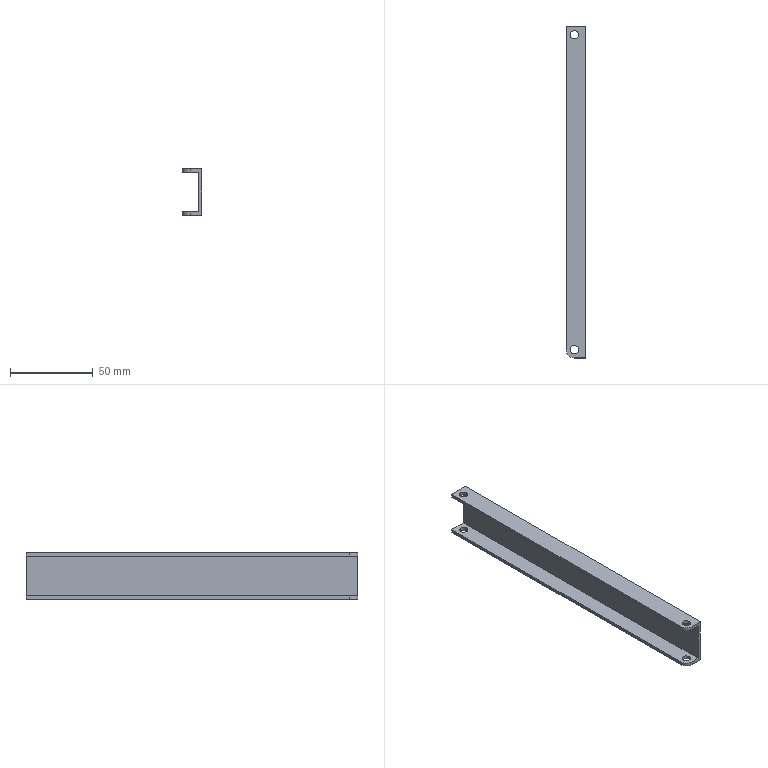Part | SolidWorks | features Cut 2, Extrusion 1, Fillet 1 | 1 solid | 20 faces | box 12 x 200 x 28 mm | volume 19021 mm3 | cylinder 10 | plane 10 | commonest cylinder face diameters 5 x8 10 x2
STEP:
#1=CARTESIAN_POINT('',(32.,242.23,-22.));
#2=VERTEX_POINT('',#1);
#3=CARTESIAN_POINT('',(32.,247.23,-22.));
#4=VERTEX_POINT('',#3);
#5=CARTESIAN_POINT('',(32.,244.73,-22.));
#6=DIRECTION('',(0.,0.,-1.));
#7=DIRECTION('',(-1.,0.,0.));
#8=AXIS2_PLACEMENT_3D('',#5,#6,#7);
#9=CIRCLE('',#8,2.5);
#10=EDGE_CURVE('',#2,#4,#9,.T.);
#11=ORIENTED_EDGE('',*,*,#10,.F.);
#12=CARTESIAN_POINT('',(32.,242.23,-24.));
#13=VERTEX_POINT('',#12);
#14=CARTESIAN_POINT('',(32.,242.23,4.));
#15=DIRECTION('',(0.,0.,-1.));
#16=VECTOR('',#15,1000.);
#17=LINE('',#14,#16);
#18=EDGE_CURVE('',#2,#13,#17,.T.);
#19=ORIENTED_EDGE('',*,*,#18,.T.);
#20=CARTESIAN_POINT('',(32.,247.23,-24.));
#21=VERTEX_POINT('',#20);
#22=CARTESIAN_POINT('',(32.,244.73,-24.));
#23=DIRECTION('',(0.,0.,-1.));
#24=DIRECTION('',(0.,1.,0.));
#25=AXIS2_PLACEMENT_3D('',#22,#23,#24);
#26=CIRCLE('',#25,2.5);
#27=EDGE_CURVE('',#13,#21,#26,.T.);
#28=ORIENTED_EDGE('',*,*,#27,.T.);
#29=CARTESIAN_POINT('',(32.,247.23,4.));
#30=DIRECTION('',(0.,0.,-1.));
#31=VECTOR('',#30,1000.);
#32=LINE('',#29,#31);
#33=EDGE_CURVE('',#4,#21,#32,.T.);
#34=ORIENTED_EDGE('',*,*,#33,.F.);
#35=EDGE_LOOP('',(#11,#19,#28,#34));
#36=FACE_OUTER_BOUND('',#35,.T.);
#37=CARTESIAN_POINT('',(32.,244.73,4.));
#38=DIRECTION('',(0.,0.,-1.));
#39=DIRECTION('',(0.,1.,0.));
#40=AXIS2_PLACEMENT_3D('',#37,#38,#39);
#41=CYLINDRICAL_SURFACE('',#40,2.5);
#42=ADVANCED_FACE('',(#36),#41,.F.);
#43=CARTESIAN_POINT('',(32.,242.23,4.));
#44=VERTEX_POINT('',#43);
#45=CARTESIAN_POINT('',(32.,247.23,4.));
#46=VERTEX_POINT('',#45);
#47=CARTESIAN_POINT('',(32.,244.73,4.));
#48=DIRECTION('',(0.,0.,-1.));
#49=DIRECTION('',(0.,1.,0.));
#50=AXIS2_PLACEMENT_3D('',#47,#48,#49);
#51=CIRCLE('',#50,2.5);
#52=EDGE_CURVE('',#44,#46,#51,.T.);
#53=ORIENTED_EDGE('',*,*,#52,.F.);
#54=CARTESIAN_POINT('',(32.,242.23,2.));
#55=VERTEX_POINT('',#54);
#56=CARTESIAN_POINT('',(32.,242.23,4.));
#57=DIRECTION('',(0.,0.,-1.));
#58=VECTOR('',#57,1000.);
#59=LINE('',#56,#58);
#60=EDGE_CURVE('',#44,#55,#59,.T.);
#61=ORIENTED_EDGE('',*,*,#60,.T.);
#62=CARTESIAN_POINT('',(32.,247.23,2.));
#63=VERTEX_POINT('',#62);
#64=CARTESIAN_POINT('',(32.,244.73,2.));
#65=DIRECTION('',(0.,0.,1.));
#66=DIRECTION('',(1.,0.,0.));
#67=AXIS2_PLACEMENT_3D('',#64,#65,#66);
#68=CIRCLE('',#67,2.5);
#69=EDGE_CURVE('',#63,#55,#68,.T.);
#70=ORIENTED_EDGE('',*,*,#69,.F.);
#71=CARTESIAN_POINT('',(32.,247.23,4.));
#72=DIRECTION('',(0.,0.,-1.));
#73=VECTOR('',#72,1000.);
#74=LINE('',#71,#73);
#75=EDGE_CURVE('',#46,#63,#74,.T.);
#76=ORIENTED_EDGE('',*,*,#75,.F.);
#77=EDGE_LOOP('',(#53,#61,#70,#76));
#78=FACE_OUTER_BOUND('',#77,.T.);
#79=CARTESIAN_POINT('',(32.,244.73,4.));
#80=DIRECTION('',(0.,0.,-1.));
#81=DIRECTION('',(0.,1.,0.));
#82=AXIS2_PLACEMENT_3D('',#79,#80,#81);
#83=CYLINDRICAL_SURFACE('',#82,2.5);
#84=ADVANCED_FACE('',(#78),#83,.F.);
#85=CARTESIAN_POINT('',(34.5,55.,-22.));
#86=VERTEX_POINT('',#85);
#87=CARTESIAN_POINT('',(29.5,55.,-22.));
#88=VERTEX_POINT('',#87);
#89=CARTESIAN_POINT('',(32.,55.,-22.));
#90=DIRECTION('',(0.,0.,-1.));
#91=DIRECTION('',(-1.,0.,0.));
#92=AXIS2_PLACEMENT_3D('',#89,#90,#91);
#93=CIRCLE('',#92,2.5);
#94=EDGE_CURVE('',#86,#88,#93,.T.);
#95=ORIENTED_EDGE('',*,*,#94,.F.);
#96=CARTESIAN_POINT('',(34.5,55.,-24.));
#97=VERTEX_POINT('',#96);
#98=CARTESIAN_POINT('',(34.5,55.,4.));
#99=DIRECTION('',(0.,0.,-1.));
#100=VECTOR('',#99,1000.);
#101=LINE('',#98,#100);
#102=EDGE_CURVE('',#86,#97,#101,.T.);
#103=ORIENTED_EDGE('',*,*,#102,.T.);
#104=CARTESIAN_POINT('',(29.5,55.,-24.));
#105=VERTEX_POINT('',#104);
#106=CARTESIAN_POINT('',(32.,55.,-24.));
#107=DIRECTION('',(0.,0.,-1.));
#108=DIRECTION('',(-1.,0.,0.));
#109=AXIS2_PLACEMENT_3D('',#106,#107,#108);
#110=CIRCLE('',#109,2.5);
#111=EDGE_CURVE('',#97,#105,#110,.T.);
#112=ORIENTED_EDGE('',*,*,#111,.T.);
#113=CARTESIAN_POINT('',(29.5,55.,4.));
#114=DIRECTION('',(0.,0.,-1.));
#115=VECTOR('',#114,1000.);
#116=LINE('',#113,#115);
#117=EDGE_CURVE('',#88,#105,#116,.T.);
#118=ORIENTED_EDGE('',*,*,#117,.F.);
#119=EDGE_LOOP('',(#95,#103,#112,#118));
#120=FACE_OUTER_BOUND('',#119,.T.);
#121=CARTESIAN_POINT('',(32.,55.,4.));
#122=DIRECTION('',(0.,0.,-1.));
#123=DIRECTION('',(-1.,0.,0.));
#124=AXIS2_PLACEMENT_3D('',#121,#122,#123);
#125=CYLINDRICAL_SURFACE('',#124,2.5);
#126=ADVANCED_FACE('',(#120),#125,.F.);
#127=CARTESIAN_POINT('',(34.5,55.,4.));
#128=VERTEX_POINT('',#127);
#129=CARTESIAN_POINT('',(29.5,55.,4.));
#130=VERTEX_POINT('',#129);
#131=CARTESIAN_POINT('',(32.,55.,4.));
#132=DIRECTION('',(0.,0.,-1.));
#133=DIRECTION('',(-1.,0.,0.));
#134=AXIS2_PLACEMENT_3D('',#131,#132,#133);
#135=CIRCLE('',#134,2.5);
#136=EDGE_CURVE('',#128,#130,#135,.T.);
#137=ORIENTED_EDGE('',*,*,#136,.F.);
#138=CARTESIAN_POINT('',(34.5,55.,2.));
#139=VERTEX_POINT('',#138);
#140=CARTESIAN_POINT('',(34.5,55.,4.));
#141=DIRECTION('',(0.,0.,-1.));
#142=VECTOR('',#141,1000.);
#143=LINE('',#140,#142);
#144=EDGE_CURVE('',#128,#139,#143,.T.);
#145=ORIENTED_EDGE('',*,*,#144,.T.);
#146=CARTESIAN_POINT('',(29.5,55.,2.));
#147=VERTEX_POINT('',#146);
#148=CARTESIAN_POINT('',(32.,55.,2.));
#149=DIRECTION('',(0.,0.,1.));
#150=DIRECTION('',(1.,0.,0.));
#151=AXIS2_PLACEMENT_3D('',#148,#149,#150);
#152=CIRCLE('',#151,2.5);
#153=EDGE_CURVE('',#147,#139,#152,.T.);
#154=ORIENTED_EDGE('',*,*,#153,.F.);
#155=CARTESIAN_POINT('',(29.5,55.,4.));
#156=DIRECTION('',(0.,0.,-1.));
#157=VECTOR('',#156,1000.);
#158=LINE('',#155,#157);
#159=EDGE_CURVE('',#130,#147,#158,.T.);
#160=ORIENTED_EDGE('',*,*,#159,.F.);
#161=EDGE_LOOP('',(#137,#145,#154,#160));
#162=FACE_OUTER_BOUND('',#161,.T.);
#163=CARTESIAN_POINT('',(32.,55.,4.));
#164=DIRECTION('',(0.,0.,-1.));
#165=DIRECTION('',(-1.,0.,0.));
#166=AXIS2_PLACEMENT_3D('',#163,#164,#165);
#167=CYLINDRICAL_SURFACE('',#166,2.5);
#168=ADVANCED_FACE('',(#162),#167,.F.);
#169=CARTESIAN_POINT('',(27.,250.,2.));
#170=VERTEX_POINT('',#169);
#171=CARTESIAN_POINT('',(27.,55.,2.));
#172=VERTEX_POINT('',#171);
#173=CARTESIAN_POINT('',(27.,250.,2.));
#174=DIRECTION('',(0.,-1.,0.));
#175=VECTOR('',#174,1000.);
#176=LINE('',#173,#175);
#177=EDGE_CURVE('',#170,#172,#176,.T.);
#178=ORIENTED_EDGE('',*,*,#177,.T.);
#179=CARTESIAN_POINT('',(27.,55.,4.));
#180=VERTEX_POINT('',#179);
#181=CARTESIAN_POINT('',(27.,55.,4.));
#182=DIRECTION('',(0.,0.,1.));
#183=VECTOR('',#182,1000.);
#184=LINE('',#181,#183);
#185=EDGE_CURVE('',#172,#180,#184,.T.);
#186=ORIENTED_EDGE('',*,*,#185,.T.);
#187=CARTESIAN_POINT('',(27.,250.,4.));
#188=VERTEX_POINT('',#187);
#189=CARTESIAN_POINT('',(27.,250.,4.));
#190=DIRECTION('',(0.,-1.,0.));
#191=VECTOR('',#190,1000.);
#192=LINE('',#189,#191);
#193=EDGE_CURVE('',#188,#180,#192,.T.);
#194=ORIENTED_EDGE('',*,*,#193,.F.);
#195=CARTESIAN_POINT('',(27.,250.,2.));
#196=DIRECTION('',(0.,0.,1.));
#197=VECTOR('',#196,1000.);
#198=LINE('',#195,#197);
#199=EDGE_CURVE('',#170,#188,#198,.T.);
#200=ORIENTED_EDGE('',*,*,#199,.F.);
#201=EDGE_LOOP('',(#178,#186,#194,#200));
#202=FACE_OUTER_BOUND('',#201,.T.);
#203=CARTESIAN_POINT('',(27.,250.,2.));
#204=DIRECTION('',(1.,0.,0.));
#205=DIRECTION('',(0.,0.,-1.));
#206=AXIS2_PLACEMENT_3D('',#203,#204,#205);
#207=PLANE('',#206);
#208=ADVANCED_FACE('',(#202),#207,.F.);
#209=CARTESIAN_POINT('',(32.,244.73,4.));
#210=DIRECTION('',(0.,0.,-1.));
#211=DIRECTION('',(0.,1.,0.));
#212=AXIS2_PLACEMENT_3D('',#209,#210,#211);
#213=CIRCLE('',#212,2.5);
#214=EDGE_CURVE('',#46,#44,#213,.T.);
#215=ORIENTED_EDGE('',*,*,#214,.T.);
#216=ORIENTED_EDGE('',*,*,#52,.T.);
#217=EDGE_LOOP('',(#215,#216));
#218=FACE_BOUND('',#217,.T.);
#219=CARTESIAN_POINT('',(32.,55.,4.));
#220=DIRECTION('',(0.,0.,-1.));
#221=DIRECTION('',(-1.,0.,0.));
#222=AXIS2_PLACEMENT_3D('',#219,#220,#221);
#223=CIRCLE('',#222,2.5);
#224=EDGE_CURVE('',#130,#128,#223,.T.);
#225=ORIENTED_EDGE('',*,*,#224,.T.);
#226=ORIENTED_EDGE('',*,*,#136,.T.);
#227=EDGE_LOOP('',(#225,#226));
#228=FACE_BOUND('',#227,.T.);
#229=ORIENTED_EDGE('',*,*,#193,.T.);
#230=CARTESIAN_POINT('',(32.,50.,4.));
#231=VERTEX_POINT('',#230);
#232=CARTESIAN_POINT('',(32.,55.,4.));
#233=DIRECTION('',(0.,0.,1.));
#234=DIRECTION('',(-1.,0.,0.));
#235=AXIS2_PLACEMENT_3D('',#232,#233,#234);
#236=CIRCLE('',#235,5.);
#237=EDGE_CURVE('',#180,#231,#236,.T.);
#238=ORIENTED_EDGE('',*,*,#237,.T.);
#239=CARTESIAN_POINT('',(39.,50.,4.));
#240=VERTEX_POINT('',#239);
#241=CARTESIAN_POINT('',(39.,50.,4.));
#242=DIRECTION('',(1.,0.,0.));
#243=VECTOR('',#242,1000.);
#244=LINE('',#241,#243);
#245=EDGE_CURVE('',#231,#240,#244,.T.);
#246=ORIENTED_EDGE('',*,*,#245,.T.);
#247=CARTESIAN_POINT('',(39.,250.,4.));
#248=VERTEX_POINT('',#247);
#249=CARTESIAN_POINT('',(39.,250.,4.));
#250=DIRECTION('',(0.,-1.,0.));
#251=VECTOR('',#250,1000.);
#252=LINE('',#249,#251);
#253=EDGE_CURVE('',#248,#240,#252,.T.);
#254=ORIENTED_EDGE('',*,*,#253,.F.);
#255=CARTESIAN_POINT('',(39.,250.,4.));
#256=DIRECTION('',(1.,0.,0.));
#257=VECTOR('',#256,1000.);
#258=LINE('',#255,#257);
#259=EDGE_CURVE('',#188,#248,#258,.T.);
#260=ORIENTED_EDGE('',*,*,#259,.F.);
#261=EDGE_LOOP('',(#229,#238,#246,#254,#260));
#262=FACE_OUTER_BOUND('',#261,.T.);
#263=CARTESIAN_POINT('',(39.,250.,4.));
#264=DIRECTION('',(0.,0.,-1.));
#265=DIRECTION('',(-1.,0.,0.));
#266=AXIS2_PLACEMENT_3D('',#263,#264,#265);
#267=PLANE('',#266);
#268=ADVANCED_FACE('',(#218,#228,#262),#267,.F.);
#269=CARTESIAN_POINT('',(39.,50.,-24.));
#270=VERTEX_POINT('',#269);
#271=CARTESIAN_POINT('',(39.,50.,-24.));
#272=DIRECTION('',(0.,0.,-1.));
#273=VECTOR('',#272,1000.);
#274=LINE('',#271,#273);
#275=EDGE_CURVE('',#240,#270,#274,.T.);
#276=ORIENTED_EDGE('',*,*,#275,.T.);
#277=CARTESIAN_POINT('',(39.,250.,-24.));
#278=VERTEX_POINT('',#277);
#279=CARTESIAN_POINT('',(39.,250.,-24.));
#280=DIRECTION('',(0.,-1.,0.));
#281=VECTOR('',#280,1000.);
#282=LINE('',#279,#281);
#283=EDGE_CURVE('',#278,#270,#282,.T.);
#284=ORIENTED_EDGE('',*,*,#283,.F.);
#285=CARTESIAN_POINT('',(39.,250.,-24.));
#286=DIRECTION('',(0.,0.,-1.));
#287=VECTOR('',#286,1000.);
#288=LINE('',#285,#287);
#289=EDGE_CURVE('',#248,#278,#288,.T.);
#290=ORIENTED_EDGE('',*,*,#289,.F.);
#291=ORIENTED_EDGE('',*,*,#253,.T.);
#292=EDGE_LOOP('',(#276,#284,#290,#291));
#293=FACE_OUTER_BOUND('',#292,.T.);
#294=CARTESIAN_POINT('',(39.,250.,-24.));
#295=DIRECTION('',(-1.,0.,0.));
#296=DIRECTION('',(0.,0.,1.));
#297=AXIS2_PLACEMENT_3D('',#294,#295,#296);
#298=PLANE('',#297);
#299=ADVANCED_FACE('',(#293),#298,.F.);
#300=CARTESIAN_POINT('',(32.,244.73,-24.));
#301=DIRECTION('',(0.,0.,-1.));
#302=DIRECTION('',(0.,1.,0.));
#303=AXIS2_PLACEMENT_3D('',#300,#301,#302);
#304=CIRCLE('',#303,2.5);
#305=EDGE_CURVE('',#21,#13,#304,.T.);
#306=ORIENTED_EDGE('',*,*,#305,.F.);
#307=ORIENTED_EDGE('',*,*,#27,.F.);
#308=EDGE_LOOP('',(#306,#307));
#309=FACE_BOUND('',#308,.T.);
#310=CARTESIAN_POINT('',(32.,55.,-24.));
#311=DIRECTION('',(0.,0.,-1.));
#312=DIRECTION('',(-1.,0.,0.));
#313=AXIS2_PLACEMENT_3D('',#310,#311,#312);
#314=CIRCLE('',#313,2.5);
#315=EDGE_CURVE('',#105,#97,#314,.T.);
#316=ORIENTED_EDGE('',*,*,#315,.F.);
#317=ORIENTED_EDGE('',*,*,#111,.F.);
#318=EDGE_LOOP('',(#316,#317));
#319=FACE_BOUND('',#318,.T.);
#320=CARTESIAN_POINT('',(32.,50.,-24.));
#321=VERTEX_POINT('',#320);
#322=CARTESIAN_POINT('',(27.,50.,-24.));
#323=DIRECTION('',(-1.,0.,0.));
#324=VECTOR('',#323,1000.);
#325=LINE('',#322,#324);
#326=EDGE_CURVE('',#270,#321,#325,.T.);
#327=ORIENTED_EDGE('',*,*,#326,.T.);
#328=CARTESIAN_POINT('',(27.,55.,-24.));
#329=VERTEX_POINT('',#328);
#330=CARTESIAN_POINT('',(32.,55.,-24.));
#331=DIRECTION('',(0.,0.,-1.));
#332=DIRECTION('',(1.,0.,0.));
#333=AXIS2_PLACEMENT_3D('',#330,#331,#332);
#334=CIRCLE('',#333,5.);
#335=EDGE_CURVE('',#321,#329,#334,.T.);
#336=ORIENTED_EDGE('',*,*,#335,.T.);
#337=CARTESIAN_POINT('',(27.,250.,-24.));
#338=VERTEX_POINT('',#337);
#339=CARTESIAN_POINT('',(27.,250.,-24.));
#340=DIRECTION('',(0.,-1.,0.));
#341=VECTOR('',#340,1000.);
#342=LINE('',#339,#341);
#343=EDGE_CURVE('',#338,#329,#342,.T.);
#344=ORIENTED_EDGE('',*,*,#343,.F.);
#345=CARTESIAN_POINT('',(27.,250.,-24.));
#346=DIRECTION('',(-1.,0.,0.));
#347=VECTOR('',#346,1000.);
#348=LINE('',#345,#347);
#349=EDGE_CURVE('',#278,#338,#348,.T.);
#350=ORIENTED_EDGE('',*,*,#349,.F.);
#351=ORIENTED_EDGE('',*,*,#283,.T.);
#352=EDGE_LOOP('',(#327,#336,#344,#350,#351));
#353=FACE_OUTER_BOUND('',#352,.T.);
#354=CARTESIAN_POINT('',(27.,250.,-24.));
#355=DIRECTION('',(0.,0.,1.));
#356=DIRECTION('',(1.,0.,0.));
#357=AXIS2_PLACEMENT_3D('',#354,#355,#356);
#358=PLANE('',#357);
#359=ADVANCED_FACE('',(#309,#319,#353),#358,.F.);
#360=ORIENTED_EDGE('',*,*,#343,.T.);
#361=CARTESIAN_POINT('',(27.,55.,-22.));
#362=VERTEX_POINT('',#361);
#363=CARTESIAN_POINT('',(27.,55.,-22.));
#364=DIRECTION('',(0.,0.,1.));
#365=VECTOR('',#364,1000.);
#366=LINE('',#363,#365);
#367=EDGE_CURVE('',#329,#362,#366,.T.);
#368=ORIENTED_EDGE('',*,*,#367,.T.);
#369=CARTESIAN_POINT('',(27.,250.,-22.));
#370=VERTEX_POINT('',#369);
#371=CARTESIAN_POINT('',(27.,250.,-22.));
#372=DIRECTION('',(0.,-1.,0.));
#373=VECTOR('',#372,1000.);
#374=LINE('',#371,#373);
#375=EDGE_CURVE('',#370,#362,#374,.T.);
#376=ORIENTED_EDGE('',*,*,#375,.F.);
#377=CARTESIAN_POINT('',(27.,250.,-22.));
#378=DIRECTION('',(0.,0.,1.));
#379=VECTOR('',#378,1000.);
#380=LINE('',#377,#379);
#381=EDGE_CURVE('',#338,#370,#380,.T.);
#382=ORIENTED_EDGE('',*,*,#381,.F.);
#383=EDGE_LOOP('',(#360,#368,#376,#382));
#384=FACE_OUTER_BOUND('',#383,.T.);
#385=CARTESIAN_POINT('',(27.,250.,-22.));
#386=DIRECTION('',(1.,0.,0.));
#387=DIRECTION('',(0.,0.,-1.));
#388=AXIS2_PLACEMENT_3D('',#385,#386,#387);
#389=PLANE('',#388);
#390=ADVANCED_FACE('',(#384),#389,.F.);
#391=CARTESIAN_POINT('',(32.,244.73,-22.));
#392=DIRECTION('',(0.,0.,-1.));
#393=DIRECTION('',(-1.,0.,0.));
#394=AXIS2_PLACEMENT_3D('',#391,#392,#393);
#395=CIRCLE('',#394,2.5);
#396=EDGE_CURVE('',#4,#2,#395,.T.);
#397=ORIENTED_EDGE('',*,*,#396,.T.);
#398=ORIENTED_EDGE('',*,*,#10,.T.);
#399=EDGE_LOOP('',(#397,#398));
#400=FACE_BOUND('',#399,.T.);
#401=CARTESIAN_POINT('',(32.,55.,-22.));
#402=DIRECTION('',(0.,0.,-1.));
#403=DIRECTION('',(-1.,0.,0.));
#404=AXIS2_PLACEMENT_3D('',#401,#402,#403);
#405=CIRCLE('',#404,2.5);
#406=EDGE_CURVE('',#88,#86,#405,.T.);
#407=ORIENTED_EDGE('',*,*,#406,.T.);
#408=ORIENTED_EDGE('',*,*,#94,.T.);
#409=EDGE_LOOP('',(#407,#408));
#410=FACE_BOUND('',#409,.T.);
#411=ORIENTED_EDGE('',*,*,#375,.T.);
#412=CARTESIAN_POINT('',(32.,50.,-22.));
#413=VERTEX_POINT('',#412);
#414=CARTESIAN_POINT('',(32.,55.,-22.));
#415=DIRECTION('',(0.,0.,1.));
#416=DIRECTION('',(-1.,0.,0.));
#417=AXIS2_PLACEMENT_3D('',#414,#415,#416);
#418=CIRCLE('',#417,5.);
#419=EDGE_CURVE('',#362,#413,#418,.T.);
#420=ORIENTED_EDGE('',*,*,#419,.T.);
#421=CARTESIAN_POINT('',(37.,50.,-22.));
#422=VERTEX_POINT('',#421);
#423=CARTESIAN_POINT('',(27.,50.,-22.));
#424=DIRECTION('',(1.,0.,0.));
#425=VECTOR('',#424,1000.);
#426=LINE('',#423,#425);
#427=EDGE_CURVE('',#413,#422,#426,.T.);
#428=ORIENTED_EDGE('',*,*,#427,.T.);
#429=CARTESIAN_POINT('',(37.,250.,-22.));
#430=VERTEX_POINT('',#429);
#431=CARTESIAN_POINT('',(37.,250.,-22.));
#432=DIRECTION('',(0.,-1.,0.));
#433=VECTOR('',#432,1000.);
#434=LINE('',#431,#433);
#435=EDGE_CURVE('',#430,#422,#434,.T.);
#436=ORIENTED_EDGE('',*,*,#435,.F.);
#437=CARTESIAN_POINT('',(27.,250.,-22.));
#438=DIRECTION('',(1.,0.,0.));
#439=VECTOR('',#438,1000.);
#440=LINE('',#437,#439);
#441=EDGE_CURVE('',#370,#430,#440,.T.);
#442=ORIENTED_EDGE('',*,*,#441,.F.);
#443=EDGE_LOOP('',(#411,#420,#428,#436,#442));
#444=FACE_OUTER_BOUND('',#443,.T.);
#445=CARTESIAN_POINT('',(27.,250.,-22.));
#446=DIRECTION('',(0.,0.,-1.));
#447=DIRECTION('',(-1.,0.,0.));
#448=AXIS2_PLACEMENT_3D('',#445,#446,#447);
#449=PLANE('',#448);
#450=ADVANCED_FACE('',(#400,#410,#444),#449,.F.);
#451=CARTESIAN_POINT('',(37.,50.,2.));
#452=VERTEX_POINT('',#451);
#453=CARTESIAN_POINT('',(37.,50.,-22.));
#454=DIRECTION('',(0.,0.,1.));
#455=VECTOR('',#454,1000.);
#456=LINE('',#453,#455);
#457=EDGE_CURVE('',#422,#452,#456,.T.);
#458=ORIENTED_EDGE('',*,*,#457,.T.);
#459=CARTESIAN_POINT('',(37.,250.,2.));
#460=VERTEX_POINT('',#459);
#461=CARTESIAN_POINT('',(37.,250.,2.));
#462=DIRECTION('',(0.,-1.,0.));
#463=VECTOR('',#462,1000.);
#464=LINE('',#461,#463);
#465=EDGE_CURVE('',#460,#452,#464,.T.);
#466=ORIENTED_EDGE('',*,*,#465,.F.);
#467=CARTESIAN_POINT('',(37.,250.,-22.));
#468=DIRECTION('',(0.,0.,1.));
#469=VECTOR('',#468,1000.);
#470=LINE('',#467,#469);
#471=EDGE_CURVE('',#430,#460,#470,.T.);
#472=ORIENTED_EDGE('',*,*,#471,.F.);
#473=ORIENTED_EDGE('',*,*,#435,.T.);
#474=EDGE_LOOP('',(#458,#466,#472,#473));
#475=FACE_OUTER_BOUND('',#474,.T.);
#476=CARTESIAN_POINT('',(37.,250.,-22.));
#477=DIRECTION('',(1.,0.,0.));
#478=DIRECTION('',(0.,0.,-1.));
#479=AXIS2_PLACEMENT_3D('',#476,#477,#478);
#480=PLANE('',#479);
#481=ADVANCED_FACE('',(#475),#480,.F.);
#482=ORIENTED_EDGE('',*,*,#69,.T.);
#483=CARTESIAN_POINT('',(32.,244.73,2.));
#484=DIRECTION('',(0.,0.,1.));
#485=DIRECTION('',(1.,0.,0.));
#486=AXIS2_PLACEMENT_3D('',#483,#484,#485);
#487=CIRCLE('',#486,2.5);
#488=EDGE_CURVE('',#55,#63,#487,.T.);
#489=ORIENTED_EDGE('',*,*,#488,.T.);
#490=EDGE_LOOP('',(#482,#489));
#491=FACE_BOUND('',#490,.T.);
#492=ORIENTED_EDGE('',*,*,#153,.T.);
#493=CARTESIAN_POINT('',(32.,55.,2.));
#494=DIRECTION('',(0.,0.,1.));
#495=DIRECTION('',(1.,0.,0.));
#496=AXIS2_PLACEMENT_3D('',#493,#494,#495);
#497=CIRCLE('',#496,2.5);
#498=EDGE_CURVE('',#139,#147,#497,.T.);
#499=ORIENTED_EDGE('',*,*,#498,.T.);
#500=EDGE_LOOP('',(#492,#499));
#501=FACE_BOUND('',#500,.T.);
#502=CARTESIAN_POINT('',(32.,50.,2.));
#503=VERTEX_POINT('',#502);
#504=CARTESIAN_POINT('',(37.,50.,2.));
#505=DIRECTION('',(-1.,0.,0.));
#506=VECTOR('',#505,1000.);
#507=LINE('',#504,#506);
#508=EDGE_CURVE('',#452,#503,#507,.T.);
#509=ORIENTED_EDGE('',*,*,#508,.T.);
#510=CARTESIAN_POINT('',(32.,55.,2.));
#511=DIRECTION('',(0.,0.,-1.));
#512=DIRECTION('',(1.,0.,0.));
#513=AXIS2_PLACEMENT_3D('',#510,#511,#512);
#514=CIRCLE('',#513,5.);
#515=EDGE_CURVE('',#503,#172,#514,.T.);
#516=ORIENTED_EDGE('',*,*,#515,.T.);
#517=ORIENTED_EDGE('',*,*,#177,.F.);
#518=CARTESIAN_POINT('',(37.,250.,2.));
#519=DIRECTION('',(-1.,0.,0.));
#520=VECTOR('',#519,1000.);
#521=LINE('',#518,#520);
#522=EDGE_CURVE('',#460,#170,#521,.T.);
#523=ORIENTED_EDGE('',*,*,#522,.F.);
#524=ORIENTED_EDGE('',*,*,#465,.T.);
#525=EDGE_LOOP('',(#509,#516,#517,#523,#524));
#526=FACE_OUTER_BOUND('',#525,.T.);
#527=CARTESIAN_POINT('',(37.,250.,2.));
#528=DIRECTION('',(0.,0.,1.));
#529=DIRECTION('',(1.,0.,0.));
#530=AXIS2_PLACEMENT_3D('',#527,#528,#529);
#531=PLANE('',#530);
#532=ADVANCED_FACE('',(#491,#501,#526),#531,.F.);
#533=ORIENTED_EDGE('',*,*,#199,.T.);
#534=ORIENTED_EDGE('',*,*,#259,.T.);
#535=ORIENTED_EDGE('',*,*,#289,.T.);
#536=ORIENTED_EDGE('',*,*,#349,.T.);
#537=ORIENTED_EDGE('',*,*,#381,.T.);
#538=ORIENTED_EDGE('',*,*,#441,.T.);
#539=ORIENTED_EDGE('',*,*,#471,.T.);
#540=ORIENTED_EDGE('',*,*,#522,.T.);
#541=EDGE_LOOP('',(#533,#534,#535,#536,#537,#538,#539,#540));
#542=FACE_OUTER_BOUND('',#541,.T.);
#543=CARTESIAN_POINT('',(0.,250.,0.));
#544=DIRECTION('',(0.,-1.,0.));
#545=DIRECTION('',(0.,0.,-1.));
#546=AXIS2_PLACEMENT_3D('',#543,#544,#545);
#547=PLANE('',#546);
#548=ADVANCED_FACE('',(#542),#547,.F.);
#549=ORIENTED_EDGE('',*,*,#245,.F.);
#550=CARTESIAN_POINT('',(32.,50.,2.));
#551=DIRECTION('',(0.,0.,-1.));
#552=VECTOR('',#551,1000.);
#553=LINE('',#550,#552);
#554=EDGE_CURVE('',#231,#503,#553,.T.);
#555=ORIENTED_EDGE('',*,*,#554,.T.);
#556=ORIENTED_EDGE('',*,*,#508,.F.);
#557=ORIENTED_EDGE('',*,*,#457,.F.);
#558=ORIENTED_EDGE('',*,*,#427,.F.);
#559=CARTESIAN_POINT('',(32.,50.,-24.));
#560=DIRECTION('',(0.,0.,-1.));
#561=VECTOR('',#560,1000.);
#562=LINE('',#559,#561);
#563=EDGE_CURVE('',#413,#321,#562,.T.);
#564=ORIENTED_EDGE('',*,*,#563,.T.);
#565=ORIENTED_EDGE('',*,*,#326,.F.);
#566=ORIENTED_EDGE('',*,*,#275,.F.);
#567=EDGE_LOOP('',(#549,#555,#556,#557,#558,#564,#565,#566));
#568=FACE_OUTER_BOUND('',#567,.T.);
#569=CARTESIAN_POINT('',(0.,50.,0.));
#570=DIRECTION('',(0.,-1.,0.));
#571=DIRECTION('',(0.,0.,-1.));
#572=AXIS2_PLACEMENT_3D('',#569,#570,#571);
#573=PLANE('',#572);
#574=ADVANCED_FACE('',(#568),#573,.T.);
#575=ORIENTED_EDGE('',*,*,#515,.F.);
#576=ORIENTED_EDGE('',*,*,#554,.F.);
#577=ORIENTED_EDGE('',*,*,#237,.F.);
#578=ORIENTED_EDGE('',*,*,#185,.F.);
#579=EDGE_LOOP('',(#575,#576,#577,#578));
#580=FACE_OUTER_BOUND('',#579,.T.);
#581=CARTESIAN_POINT('',(32.,55.,2.));
#582=DIRECTION('',(0.,0.,-1.));
#583=DIRECTION('',(-1.,0.,0.));
#584=AXIS2_PLACEMENT_3D('',#581,#582,#583);
#585=CYLINDRICAL_SURFACE('',#584,5.);
#586=ADVANCED_FACE('',(#580),#585,.T.);
#587=ORIENTED_EDGE('',*,*,#335,.F.);
#588=ORIENTED_EDGE('',*,*,#563,.F.);
#589=ORIENTED_EDGE('',*,*,#419,.F.);
#590=ORIENTED_EDGE('',*,*,#367,.F.);
#591=EDGE_LOOP('',(#587,#588,#589,#590));
#592=FACE_OUTER_BOUND('',#591,.T.);
#593=CARTESIAN_POINT('',(32.,55.,-22.));
#594=DIRECTION('',(0.,0.,-1.));
#595=DIRECTION('',(-1.,0.,0.));
#596=AXIS2_PLACEMENT_3D('',#593,#594,#595);
#597=CYLINDRICAL_SURFACE('',#596,5.);
#598=ADVANCED_FACE('',(#592),#597,.T.);
#599=ORIENTED_EDGE('',*,*,#144,.F.);
#600=ORIENTED_EDGE('',*,*,#224,.F.);
#601=ORIENTED_EDGE('',*,*,#159,.T.);
#602=ORIENTED_EDGE('',*,*,#498,.F.);
#603=EDGE_LOOP('',(#599,#600,#601,#602));
#604=FACE_OUTER_BOUND('',#603,.T.);
#605=CARTESIAN_POINT('',(32.,55.,4.));
#606=DIRECTION('',(0.,0.,-1.));
#607=DIRECTION('',(-1.,0.,0.));
#608=AXIS2_PLACEMENT_3D('',#605,#606,#607);
#609=CYLINDRICAL_SURFACE('',#608,2.5);
#610=ADVANCED_FACE('',(#604),#609,.F.);
#611=ORIENTED_EDGE('',*,*,#102,.F.);
#612=ORIENTED_EDGE('',*,*,#406,.F.);
#613=ORIENTED_EDGE('',*,*,#117,.T.);
#614=ORIENTED_EDGE('',*,*,#315,.T.);
#615=EDGE_LOOP('',(#611,#612,#613,#614));
#616=FACE_OUTER_BOUND('',#615,.T.);
#617=CARTESIAN_POINT('',(32.,55.,4.));
#618=DIRECTION('',(0.,0.,-1.));
#619=DIRECTION('',(-1.,0.,0.));
#620=AXIS2_PLACEMENT_3D('',#617,#618,#619);
#621=CYLINDRICAL_SURFACE('',#620,2.5);
#622=ADVANCED_FACE('',(#616),#621,.F.);
#623=ORIENTED_EDGE('',*,*,#60,.F.);
#624=ORIENTED_EDGE('',*,*,#214,.F.);
#625=ORIENTED_EDGE('',*,*,#75,.T.);
#626=ORIENTED_EDGE('',*,*,#488,.F.);
#627=EDGE_LOOP('',(#623,#624,#625,#626));
#628=FACE_OUTER_BOUND('',#627,.T.);
#629=CARTESIAN_POINT('',(32.,244.73,4.));
#630=DIRECTION('',(0.,0.,-1.));
#631=DIRECTION('',(0.,1.,0.));
#632=AXIS2_PLACEMENT_3D('',#629,#630,#631);
#633=CYLINDRICAL_SURFACE('',#632,2.5);
#634=ADVANCED_FACE('',(#628),#633,.F.);
#635=ORIENTED_EDGE('',*,*,#18,.F.);
#636=ORIENTED_EDGE('',*,*,#396,.F.);
#637=ORIENTED_EDGE('',*,*,#33,.T.);
#638=ORIENTED_EDGE('',*,*,#305,.T.);
#639=EDGE_LOOP('',(#635,#636,#637,#638));
#640=FACE_OUTER_BOUND('',#639,.T.);
#641=CARTESIAN_POINT('',(32.,244.73,4.));
#642=DIRECTION('',(0.,0.,-1.));
#643=DIRECTION('',(0.,1.,0.));
#644=AXIS2_PLACEMENT_3D('',#641,#642,#643);
#645=CYLINDRICAL_SURFACE('',#644,2.5);
#646=ADVANCED_FACE('',(#640),#645,.F.);
#647=CLOSED_SHELL('',(#42,#84,#126,#168,#208,#268,#299,#359,#390,#450,#481,#532,#548,#574,#586,#598,#610,#622,#634,#646));
#648=MANIFOLD_SOLID_BREP('',#647);
#649=CARTESIAN_POINT('',(0.,0.,0.));
#650=DIRECTION('',(0.,0.,1.));
#651=DIRECTION('',(1.,0.,0.));
#652=AXIS2_PLACEMENT_3D('',#649,#650,#651);
#653=(LENGTH_UNIT()NAMED_UNIT(*)SI_UNIT(.MILLI.,.METRE.));
#654=UNCERTAINTY_MEASURE_WITH_UNIT(LENGTH_MEASURE(0.00001),#653,'','');
#655=(NAMED_UNIT(*)PLANE_ANGLE_UNIT()SI_UNIT($,.RADIAN.));
#656=(NAMED_UNIT(*)SI_UNIT($,.STERADIAN.)SOLID_ANGLE_UNIT());
#657=(GEOMETRIC_REPRESENTATION_CONTEXT(3)GLOBAL_UNCERTAINTY_ASSIGNED_CONTEXT((#654))GLOBAL_UNIT_ASSIGNED_CONTEXT((#653,#655,#656))REPRESENTATION_CONTEXT('',''));
#658=ADVANCED_BREP_SHAPE_REPRESENTATION('',(#648,#652),#657);